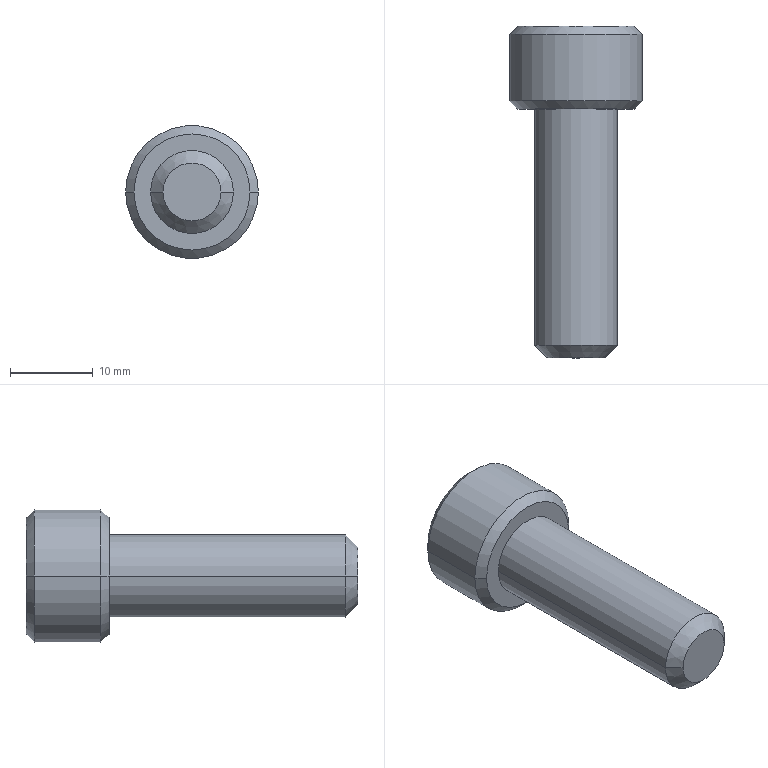Part | STEP file | BB62-M10-30L-9 | 1 solid | 27 faces | box 16 x 40 x 16 mm | volume 3957 mm3 | plane 15 | cone 8 | cylinder 4 | commonest cylinder face diameters 10 x2 16 x2
STEP:
#1=CARTESIAN_POINT('',(0.,2.359,0.));
#2=VERTEX_POINT('',#1);
#3=CARTESIAN_POINT('',(4.575,5.,0.));
#4=VERTEX_POINT('',#3);
#5=CARTESIAN_POINT('',(0.,2.359,0.));
#6=DIRECTION('',(0.866,0.5,0.));
#7=VECTOR('',#6,1000.);
#8=LINE('',#5,#7);
#9=EDGE_CURVE('',#2,#4,#8,.T.);
#10=ORIENTED_EDGE('',*,*,#9,.F.);
#11=CARTESIAN_POINT('',(-4.575,5.,0.));
#12=VERTEX_POINT('',#11);
#13=CARTESIAN_POINT('',(0.,2.359,0.));
#14=DIRECTION('',(-0.866,0.5,0.));
#15=VECTOR('',#14,1000.);
#16=LINE('',#13,#15);
#17=EDGE_CURVE('',#2,#12,#16,.T.);
#18=ORIENTED_EDGE('',*,*,#17,.T.);
#19=CARTESIAN_POINT('',(-3.962,5.,2.288));
#20=VERTEX_POINT('',#19);
#21=CARTESIAN_POINT('',(0.,5.,0.));
#22=DIRECTION('',(0.,-1.,0.));
#23=DIRECTION('',(-1.,0.,0.));
#24=AXIS2_PLACEMENT_3D('',#21,#22,#23);
#25=CIRCLE('',#24,4.575);
#26=EDGE_CURVE('',#20,#12,#25,.T.);
#27=ORIENTED_EDGE('',*,*,#26,.F.);
#28=CARTESIAN_POINT('',(0.,5.,4.575));
#29=VERTEX_POINT('',#28);
#30=CARTESIAN_POINT('',(0.,5.,0.));
#31=DIRECTION('',(0.,-1.,0.));
#32=DIRECTION('',(-1.,0.,0.));
#33=AXIS2_PLACEMENT_3D('',#30,#31,#32);
#34=CIRCLE('',#33,4.575);
#35=EDGE_CURVE('',#29,#20,#34,.T.);
#36=ORIENTED_EDGE('',*,*,#35,.F.);
#37=CARTESIAN_POINT('',(3.962,5.,2.287));
#38=VERTEX_POINT('',#37);
#39=CARTESIAN_POINT('',(0.,5.,0.));
#40=DIRECTION('',(0.,-1.,0.));
#41=DIRECTION('',(-1.,0.,0.));
#42=AXIS2_PLACEMENT_3D('',#39,#40,#41);
#43=CIRCLE('',#42,4.575);
#44=EDGE_CURVE('',#38,#29,#43,.T.);
#45=ORIENTED_EDGE('',*,*,#44,.F.);
#46=CARTESIAN_POINT('',(0.,5.,0.));
#47=DIRECTION('',(0.,-1.,0.));
#48=DIRECTION('',(-1.,0.,0.));
#49=AXIS2_PLACEMENT_3D('',#46,#47,#48);
#50=CIRCLE('',#49,4.575);
#51=EDGE_CURVE('',#4,#38,#50,.T.);
#52=ORIENTED_EDGE('',*,*,#51,.F.);
#53=EDGE_LOOP('',(#10,#18,#27,#36,#45,#52));
#54=FACE_OUTER_BOUND('',#53,.T.);
#55=CARTESIAN_POINT('',(0.,1002.359,0.));
#56=DIRECTION('',(0.,1.,0.));
#57=DIRECTION('',(1.,0.,0.));
#58=AXIS2_PLACEMENT_3D('',#55,#56,#57);
#59=CONICAL_SURFACE('',#58,1732.051,1.047);
#60=ADVANCED_FACE('',(#54),#59,.F.);
#61=CARTESIAN_POINT('',(3.5,-30.,0.));
#62=VERTEX_POINT('',#61);
#63=CARTESIAN_POINT('',(-3.5,-30.,0.));
#64=VERTEX_POINT('',#63);
#65=CARTESIAN_POINT('',(0.,-30.,0.));
#66=DIRECTION('',(0.,1.,0.));
#67=DIRECTION('',(1.,0.,0.));
#68=AXIS2_PLACEMENT_3D('',#65,#66,#67);
#69=CIRCLE('',#68,3.5);
#70=EDGE_CURVE('',#62,#64,#69,.T.);
#71=ORIENTED_EDGE('',*,*,#70,.T.);
#72=CARTESIAN_POINT('',(-5.,-28.5,0.));
#73=VERTEX_POINT('',#72);
#74=CARTESIAN_POINT('',(-3.5,-30.,0.));
#75=DIRECTION('',(-0.7071,0.7071,0.));
#76=VECTOR('',#75,1000.);
#77=LINE('',#74,#76);
#78=EDGE_CURVE('',#64,#73,#77,.T.);
#79=ORIENTED_EDGE('',*,*,#78,.T.);
#80=CARTESIAN_POINT('',(5.,-28.5,0.));
#81=VERTEX_POINT('',#80);
#82=CARTESIAN_POINT('',(0.,-28.5,0.));
#83=DIRECTION('',(0.,-1.,0.));
#84=DIRECTION('',(-1.,0.,0.));
#85=AXIS2_PLACEMENT_3D('',#82,#83,#84);
#86=CIRCLE('',#85,5.);
#87=EDGE_CURVE('',#73,#81,#86,.T.);
#88=ORIENTED_EDGE('',*,*,#87,.T.);
#89=CARTESIAN_POINT('',(3.5,-30.,0.));
#90=DIRECTION('',(0.7071,0.7071,0.));
#91=VECTOR('',#90,1000.);
#92=LINE('',#89,#91);
#93=EDGE_CURVE('',#62,#81,#92,.T.);
#94=ORIENTED_EDGE('',*,*,#93,.F.);
#95=EDGE_LOOP('',(#71,#79,#88,#94));
#96=FACE_OUTER_BOUND('',#95,.T.);
#97=CARTESIAN_POINT('',(0.,-30.,0.));
#98=DIRECTION('',(0.,1.,0.));
#99=DIRECTION('',(1.,0.,0.));
#100=AXIS2_PLACEMENT_3D('',#97,#98,#99);
#101=CONICAL_SURFACE('',#100,3.5,0.7854);
#102=ADVANCED_FACE('',(#96),#101,.T.);
#103=ORIENTED_EDGE('',*,*,#87,.F.);
#104=CARTESIAN_POINT('',(-5.,0.,0.));
#105=VERTEX_POINT('',#104);
#106=CARTESIAN_POINT('',(-5.,-28.5,0.));
#107=DIRECTION('',(0.,1.,0.));
#108=VECTOR('',#107,1000.);
#109=LINE('',#106,#108);
#110=EDGE_CURVE('',#73,#105,#109,.T.);
#111=ORIENTED_EDGE('',*,*,#110,.T.);
#112=CARTESIAN_POINT('',(5.,0.,0.));
#113=VERTEX_POINT('',#112);
#114=CARTESIAN_POINT('',(0.,0.,0.));
#115=DIRECTION('',(0.,-1.,0.));
#116=DIRECTION('',(-1.,0.,0.));
#117=AXIS2_PLACEMENT_3D('',#114,#115,#116);
#118=CIRCLE('',#117,5.);
#119=EDGE_CURVE('',#105,#113,#118,.T.);
#120=ORIENTED_EDGE('',*,*,#119,.T.);
#121=CARTESIAN_POINT('',(5.,-28.5,0.));
#122=DIRECTION('',(0.,1.,0.));
#123=VECTOR('',#122,1000.);
#124=LINE('',#121,#123);
#125=EDGE_CURVE('',#81,#113,#124,.T.);
#126=ORIENTED_EDGE('',*,*,#125,.F.);
#127=EDGE_LOOP('',(#103,#111,#120,#126));
#128=FACE_OUTER_BOUND('',#127,.T.);
#129=CARTESIAN_POINT('',(0.,-28.5,0.));
#130=DIRECTION('',(0.,1.,0.));
#131=DIRECTION('',(1.,0.,0.));
#132=AXIS2_PLACEMENT_3D('',#129,#130,#131);
#133=CYLINDRICAL_SURFACE('',#132,5.);
#134=ADVANCED_FACE('',(#128),#133,.T.);
#135=CARTESIAN_POINT('',(-7.,10.,0.));
#136=VERTEX_POINT('',#135);
#137=CARTESIAN_POINT('',(7.,10.,0.));
#138=VERTEX_POINT('',#137);
#139=CARTESIAN_POINT('',(0.,10.,0.));
#140=DIRECTION('',(0.,-1.,0.));
#141=DIRECTION('',(-1.,0.,0.));
#142=AXIS2_PLACEMENT_3D('',#139,#140,#141);
#143=CIRCLE('',#142,7.);
#144=EDGE_CURVE('',#136,#138,#143,.T.);
#145=ORIENTED_EDGE('',*,*,#144,.T.);
#146=CARTESIAN_POINT('',(8.,9.,0.));
#147=VERTEX_POINT('',#146);
#148=CARTESIAN_POINT('',(8.,9.,0.));
#149=DIRECTION('',(0.7071,-0.7071,0.));
#150=VECTOR('',#149,1000.);
#151=LINE('',#148,#150);
#152=EDGE_CURVE('',#138,#147,#151,.T.);
#153=ORIENTED_EDGE('',*,*,#152,.T.);
#154=CARTESIAN_POINT('',(-8.,9.,0.));
#155=VERTEX_POINT('',#154);
#156=CARTESIAN_POINT('',(0.,9.,0.));
#157=DIRECTION('',(0.,-1.,0.));
#158=DIRECTION('',(-1.,0.,0.));
#159=AXIS2_PLACEMENT_3D('',#156,#157,#158);
#160=CIRCLE('',#159,8.);
#161=EDGE_CURVE('',#155,#147,#160,.T.);
#162=ORIENTED_EDGE('',*,*,#161,.F.);
#163=CARTESIAN_POINT('',(-8.,9.,0.));
#164=DIRECTION('',(-0.7071,-0.7071,0.));
#165=VECTOR('',#164,1000.);
#166=LINE('',#163,#165);
#167=EDGE_CURVE('',#136,#155,#166,.T.);
#168=ORIENTED_EDGE('',*,*,#167,.F.);
#169=EDGE_LOOP('',(#145,#153,#162,#168));
#170=FACE_OUTER_BOUND('',#169,.T.);
#171=CARTESIAN_POINT('',(0.,9.,0.));
#172=DIRECTION('',(0.,-1.,0.));
#173=DIRECTION('',(-1.,0.,0.));
#174=AXIS2_PLACEMENT_3D('',#171,#172,#173);
#175=CONICAL_SURFACE('',#174,8.,0.7854);
#176=ADVANCED_FACE('',(#170),#175,.T.);
#177=ORIENTED_EDGE('',*,*,#161,.T.);
#178=CARTESIAN_POINT('',(8.,1.,0.));
#179=VERTEX_POINT('',#178);
#180=CARTESIAN_POINT('',(8.,1.62,0.));
#181=DIRECTION('',(0.,-1.,0.));
#182=VECTOR('',#181,1000.);
#183=LINE('',#180,#182);
#184=EDGE_CURVE('',#147,#179,#183,.T.);
#185=ORIENTED_EDGE('',*,*,#184,.T.);
#186=CARTESIAN_POINT('',(-8.,1.,0.));
#187=VERTEX_POINT('',#186);
#188=CARTESIAN_POINT('',(0.,1.,0.));
#189=DIRECTION('',(0.,-1.,0.));
#190=DIRECTION('',(-1.,0.,0.));
#191=AXIS2_PLACEMENT_3D('',#188,#189,#190);
#192=CIRCLE('',#191,8.);
#193=EDGE_CURVE('',#187,#179,#192,.T.);
#194=ORIENTED_EDGE('',*,*,#193,.F.);
#195=CARTESIAN_POINT('',(-8.,1.62,0.));
#196=DIRECTION('',(0.,-1.,0.));
#197=VECTOR('',#196,1000.);
#198=LINE('',#195,#197);
#199=EDGE_CURVE('',#155,#187,#198,.T.);
#200=ORIENTED_EDGE('',*,*,#199,.F.);
#201=EDGE_LOOP('',(#177,#185,#194,#200));
#202=FACE_OUTER_BOUND('',#201,.T.);
#203=CARTESIAN_POINT('',(0.,1.62,0.));
#204=DIRECTION('',(0.,-1.,0.));
#205=DIRECTION('',(-1.,0.,0.));
#206=AXIS2_PLACEMENT_3D('',#203,#204,#205);
#207=CYLINDRICAL_SURFACE('',#206,8.);
#208=ADVANCED_FACE('',(#202),#207,.T.);
#209=CARTESIAN_POINT('',(-7.,0.,0.));
#210=VERTEX_POINT('',#209);
#211=CARTESIAN_POINT('',(7.,0.,0.));
#212=VERTEX_POINT('',#211);
#213=CARTESIAN_POINT('',(0.,0.,0.));
#214=DIRECTION('',(0.,-1.,0.));
#215=DIRECTION('',(-1.,0.,0.));
#216=AXIS2_PLACEMENT_3D('',#213,#214,#215);
#217=CIRCLE('',#216,7.);
#218=EDGE_CURVE('',#210,#212,#217,.T.);
#219=ORIENTED_EDGE('',*,*,#218,.F.);
#220=CARTESIAN_POINT('',(-7.,0.,0.));
#221=DIRECTION('',(-0.7071,0.7071,0.));
#222=VECTOR('',#221,1000.);
#223=LINE('',#220,#222);
#224=EDGE_CURVE('',#210,#187,#223,.T.);
#225=ORIENTED_EDGE('',*,*,#224,.T.);
#226=ORIENTED_EDGE('',*,*,#193,.T.);
#227=CARTESIAN_POINT('',(7.,0.,0.));
#228=DIRECTION('',(0.7071,0.7071,0.));
#229=VECTOR('',#228,1000.);
#230=LINE('',#227,#229);
#231=EDGE_CURVE('',#212,#179,#230,.T.);
#232=ORIENTED_EDGE('',*,*,#231,.F.);
#233=EDGE_LOOP('',(#219,#225,#226,#232));
#234=FACE_OUTER_BOUND('',#233,.T.);
#235=CARTESIAN_POINT('',(0.,0.,0.));
#236=DIRECTION('',(0.,1.,0.));
#237=DIRECTION('',(1.,0.,0.));
#238=AXIS2_PLACEMENT_3D('',#235,#236,#237);
#239=CONICAL_SURFACE('',#238,7.,0.7854);
#240=ADVANCED_FACE('',(#234),#239,.T.);
#241=ORIENTED_EDGE('',*,*,#144,.F.);
#242=CARTESIAN_POINT('',(0.,10.,0.));
#243=DIRECTION('',(0.,-1.,0.));
#244=DIRECTION('',(-1.,0.,0.));
#245=AXIS2_PLACEMENT_3D('',#242,#243,#244);
#246=CIRCLE('',#245,7.);
#247=EDGE_CURVE('',#138,#136,#246,.T.);
#248=ORIENTED_EDGE('',*,*,#247,.F.);
#249=EDGE_LOOP('',(#241,#248));
#250=FACE_OUTER_BOUND('',#249,.T.);
#251=CARTESIAN_POINT('',(0.,10.,-4.575));
#252=VERTEX_POINT('',#251);
#253=CARTESIAN_POINT('',(-3.962,10.,-2.288));
#254=VERTEX_POINT('',#253);
#255=CARTESIAN_POINT('',(0.,10.,-4.575));
#256=DIRECTION('',(-0.866,0.,0.5));
#257=VECTOR('',#256,1000.);
#258=LINE('',#255,#257);
#259=EDGE_CURVE('',#252,#254,#258,.T.);
#260=ORIENTED_EDGE('',*,*,#259,.F.);
#261=CARTESIAN_POINT('',(3.962,10.,-2.288));
#262=VERTEX_POINT('',#261);
#263=CARTESIAN_POINT('',(3.962,10.,-2.288));
#264=DIRECTION('',(-0.866,0.,-0.5));
#265=VECTOR('',#264,1000.);
#266=LINE('',#263,#265);
#267=EDGE_CURVE('',#262,#252,#266,.T.);
#268=ORIENTED_EDGE('',*,*,#267,.F.);
#269=CARTESIAN_POINT('',(3.962,10.,2.287));
#270=VERTEX_POINT('',#269);
#271=CARTESIAN_POINT('',(3.962,10.,2.287));
#272=DIRECTION('',(0.,0.,-1.));
#273=VECTOR('',#272,1000.);
#274=LINE('',#271,#273);
#275=EDGE_CURVE('',#270,#262,#274,.T.);
#276=ORIENTED_EDGE('',*,*,#275,.F.);
#277=CARTESIAN_POINT('',(0.,10.,4.575));
#278=VERTEX_POINT('',#277);
#279=CARTESIAN_POINT('',(0.,10.,4.575));
#280=DIRECTION('',(0.866,0.,-0.5));
#281=VECTOR('',#280,1000.);
#282=LINE('',#279,#281);
#283=EDGE_CURVE('',#278,#270,#282,.T.);
#284=ORIENTED_EDGE('',*,*,#283,.F.);
#285=CARTESIAN_POINT('',(-3.962,10.,2.287));
#286=VERTEX_POINT('',#285);
#287=CARTESIAN_POINT('',(-3.962,10.,2.287));
#288=DIRECTION('',(0.866,0.,0.5));
#289=VECTOR('',#288,1000.);
#290=LINE('',#287,#289);
#291=EDGE_CURVE('',#286,#278,#290,.T.);
#292=ORIENTED_EDGE('',*,*,#291,.F.);
#293=CARTESIAN_POINT('',(-3.962,10.,-2.288));
#294=DIRECTION('',(0.,0.,1.));
#295=VECTOR('',#294,1000.);
#296=LINE('',#293,#295);
#297=EDGE_CURVE('',#254,#286,#296,.T.);
#298=ORIENTED_EDGE('',*,*,#297,.F.);
#299=EDGE_LOOP('',(#260,#268,#276,#284,#292,#298));
#300=FACE_BOUND('',#299,.T.);
#301=CARTESIAN_POINT('',(7.,10.,0.));
#302=DIRECTION('',(0.,1.,0.));
#303=DIRECTION('',(1.,0.,0.));
#304=AXIS2_PLACEMENT_3D('',#301,#302,#303);
#305=PLANE('',#304);
#306=ADVANCED_FACE('',(#250,#300),#305,.T.);
#307=CARTESIAN_POINT('',(0.,0.,0.));
#308=DIRECTION('',(0.,-1.,0.));
#309=DIRECTION('',(-1.,0.,0.));
#310=AXIS2_PLACEMENT_3D('',#307,#308,#309);
#311=CIRCLE('',#310,5.);
#312=EDGE_CURVE('',#113,#105,#311,.T.);
#313=ORIENTED_EDGE('',*,*,#312,.F.);
#314=ORIENTED_EDGE('',*,*,#119,.F.);
#315=EDGE_LOOP('',(#313,#314));
#316=FACE_BOUND('',#315,.T.);
#317=CARTESIAN_POINT('',(0.,0.,0.));
#318=DIRECTION('',(0.,-1.,0.));
#319=DIRECTION('',(-1.,0.,0.));
#320=AXIS2_PLACEMENT_3D('',#317,#318,#319);
#321=CIRCLE('',#320,7.);
#322=EDGE_CURVE('',#212,#210,#321,.T.);
#323=ORIENTED_EDGE('',*,*,#322,.T.);
#324=ORIENTED_EDGE('',*,*,#218,.T.);
#325=EDGE_LOOP('',(#323,#324));
#326=FACE_OUTER_BOUND('',#325,.T.);
#327=CARTESIAN_POINT('',(0.,0.,0.));
#328=DIRECTION('',(0.,-1.,0.));
#329=DIRECTION('',(-1.,0.,0.));
#330=AXIS2_PLACEMENT_3D('',#327,#328,#329);
#331=PLANE('',#330);
#332=ADVANCED_FACE('',(#316,#326),#331,.T.);
#333=ORIENTED_EDGE('',*,*,#224,.F.);
#334=ORIENTED_EDGE('',*,*,#322,.F.);
#335=ORIENTED_EDGE('',*,*,#231,.T.);
#336=CARTESIAN_POINT('',(0.,1.,0.));
#337=DIRECTION('',(0.,-1.,0.));
#338=DIRECTION('',(-1.,0.,0.));
#339=AXIS2_PLACEMENT_3D('',#336,#337,#338);
#340=CIRCLE('',#339,8.);
#341=EDGE_CURVE('',#179,#187,#340,.T.);
#342=ORIENTED_EDGE('',*,*,#341,.T.);
#343=EDGE_LOOP('',(#333,#334,#335,#342));
#344=FACE_OUTER_BOUND('',#343,.T.);
#345=CARTESIAN_POINT('',(0.,0.,0.));
#346=DIRECTION('',(0.,1.,0.));
#347=DIRECTION('',(1.,0.,0.));
#348=AXIS2_PLACEMENT_3D('',#345,#346,#347);
#349=CONICAL_SURFACE('',#348,7.,0.7854);
#350=ADVANCED_FACE('',(#344),#349,.T.);
#351=ORIENTED_EDGE('',*,*,#184,.F.);
#352=CARTESIAN_POINT('',(0.,9.,0.));
#353=DIRECTION('',(0.,-1.,0.));
#354=DIRECTION('',(-1.,0.,0.));
#355=AXIS2_PLACEMENT_3D('',#352,#353,#354);
#356=CIRCLE('',#355,8.);
#357=EDGE_CURVE('',#147,#155,#356,.T.);
#358=ORIENTED_EDGE('',*,*,#357,.T.);
#359=ORIENTED_EDGE('',*,*,#199,.T.);
#360=ORIENTED_EDGE('',*,*,#341,.F.);
#361=EDGE_LOOP('',(#351,#358,#359,#360));
#362=FACE_OUTER_BOUND('',#361,.T.);
#363=CARTESIAN_POINT('',(0.,1.62,0.));
#364=DIRECTION('',(0.,-1.,0.));
#365=DIRECTION('',(-1.,0.,0.));
#366=AXIS2_PLACEMENT_3D('',#363,#364,#365);
#367=CYLINDRICAL_SURFACE('',#366,8.);
#368=ADVANCED_FACE('',(#362),#367,.T.);
#369=ORIENTED_EDGE('',*,*,#152,.F.);
#370=ORIENTED_EDGE('',*,*,#247,.T.);
#371=ORIENTED_EDGE('',*,*,#167,.T.);
#372=ORIENTED_EDGE('',*,*,#357,.F.);
#373=EDGE_LOOP('',(#369,#370,#371,#372));
#374=FACE_OUTER_BOUND('',#373,.T.);
#375=CARTESIAN_POINT('',(0.,9.,0.));
#376=DIRECTION('',(0.,-1.,0.));
#377=DIRECTION('',(-1.,0.,0.));
#378=AXIS2_PLACEMENT_3D('',#375,#376,#377);
#379=CONICAL_SURFACE('',#378,8.,0.7854);
#380=ADVANCED_FACE('',(#374),#379,.T.);
#381=ORIENTED_EDGE('',*,*,#110,.F.);
#382=CARTESIAN_POINT('',(0.,-28.5,0.));
#383=DIRECTION('',(0.,-1.,0.));
#384=DIRECTION('',(-1.,0.,0.));
#385=AXIS2_PLACEMENT_3D('',#382,#383,#384);
#386=CIRCLE('',#385,5.);
#387=EDGE_CURVE('',#81,#73,#386,.T.);
#388=ORIENTED_EDGE('',*,*,#387,.F.);
#389=ORIENTED_EDGE('',*,*,#125,.T.);
#390=ORIENTED_EDGE('',*,*,#312,.T.);
#391=EDGE_LOOP('',(#381,#388,#389,#390));
#392=FACE_OUTER_BOUND('',#391,.T.);
#393=CARTESIAN_POINT('',(0.,-28.5,0.));
#394=DIRECTION('',(0.,1.,0.));
#395=DIRECTION('',(1.,0.,0.));
#396=AXIS2_PLACEMENT_3D('',#393,#394,#395);
#397=CYLINDRICAL_SURFACE('',#396,5.);
#398=ADVANCED_FACE('',(#392),#397,.T.);
#399=ORIENTED_EDGE('',*,*,#70,.F.);
#400=CARTESIAN_POINT('',(0.,-30.,0.));
#401=DIRECTION('',(0.,1.,0.));
#402=DIRECTION('',(1.,0.,0.));
#403=AXIS2_PLACEMENT_3D('',#400,#401,#402);
#404=CIRCLE('',#403,3.5);
#405=EDGE_CURVE('',#64,#62,#404,.T.);
#406=ORIENTED_EDGE('',*,*,#405,.F.);
#407=EDGE_LOOP('',(#399,#406));
#408=FACE_OUTER_BOUND('',#407,.T.);
#409=CARTESIAN_POINT('',(0.,-30.,0.));
#410=DIRECTION('',(0.,-1.,0.));
#411=DIRECTION('',(-1.,0.,0.));
#412=AXIS2_PLACEMENT_3D('',#409,#410,#411);
#413=PLANE('',#412);
#414=ADVANCED_FACE('',(#408),#413,.T.);
#415=ORIENTED_EDGE('',*,*,#78,.F.);
#416=ORIENTED_EDGE('',*,*,#405,.T.);
#417=ORIENTED_EDGE('',*,*,#93,.T.);
#418=ORIENTED_EDGE('',*,*,#387,.T.);
#419=EDGE_LOOP('',(#415,#416,#417,#418));
#420=FACE_OUTER_BOUND('',#419,.T.);
#421=CARTESIAN_POINT('',(0.,-30.,0.));
#422=DIRECTION('',(0.,1.,0.));
#423=DIRECTION('',(1.,0.,0.));
#424=AXIS2_PLACEMENT_3D('',#421,#422,#423);
#425=CONICAL_SURFACE('',#424,3.5,0.7854);
#426=ADVANCED_FACE('',(#420),#425,.T.);
#427=CARTESIAN_POINT('',(3.962,5.,-2.288));
#428=VERTEX_POINT('',#427);
#429=CARTESIAN_POINT('',(0.,5.,-4.575));
#430=VERTEX_POINT('',#429);
#431=CARTESIAN_POINT('',(3.962,5.,-2.288));
#432=DIRECTION('',(-0.866,0.,-0.5));
#433=VECTOR('',#432,1000.);
#434=LINE('',#431,#433);
#435=EDGE_CURVE('',#428,#430,#434,.T.);
#436=ORIENTED_EDGE('',*,*,#435,.F.);
#437=CARTESIAN_POINT('',(3.962,10.,-2.288));
#438=DIRECTION('',(0.,-1.,0.));
#439=VECTOR('',#438,1000.);
#440=LINE('',#437,#439);
#441=EDGE_CURVE('',#262,#428,#440,.T.);
#442=ORIENTED_EDGE('',*,*,#441,.F.);
#443=ORIENTED_EDGE('',*,*,#267,.T.);
#444=CARTESIAN_POINT('',(0.,10.,-4.575));
#445=DIRECTION('',(0.,-1.,0.));
#446=VECTOR('',#445,1000.);
#447=LINE('',#444,#446);
#448=EDGE_CURVE('',#252,#430,#447,.T.);
#449=ORIENTED_EDGE('',*,*,#448,.T.);
#450=EDGE_LOOP('',(#436,#442,#443,#449));
#451=FACE_OUTER_BOUND('',#450,.T.);
#452=CARTESIAN_POINT('',(3.962,10.,-2.288));
#453=DIRECTION('',(-0.5,0.,0.866));
#454=DIRECTION('',(0.866,0.,0.5));
#455=AXIS2_PLACEMENT_3D('',#452,#453,#454);
#456=PLANE('',#455);
#457=ADVANCED_FACE('',(#451),#456,.T.);
#458=CARTESIAN_POINT('',(-3.962,5.,-2.288));
#459=VERTEX_POINT('',#458);
#460=CARTESIAN_POINT('',(0.,5.,-4.575));
#461=DIRECTION('',(-0.866,0.,0.5));
#462=VECTOR('',#461,1000.);
#463=LINE('',#460,#462);
#464=EDGE_CURVE('',#430,#459,#463,.T.);
#465=ORIENTED_EDGE('',*,*,#464,.F.);
#466=ORIENTED_EDGE('',*,*,#448,.F.);
#467=ORIENTED_EDGE('',*,*,#259,.T.);
#468=CARTESIAN_POINT('',(-3.962,10.,-2.288));
#469=DIRECTION('',(0.,-1.,0.));
#470=VECTOR('',#469,1000.);
#471=LINE('',#468,#470);
#472=EDGE_CURVE('',#254,#459,#471,.T.);
#473=ORIENTED_EDGE('',*,*,#472,.T.);
#474=EDGE_LOOP('',(#465,#466,#467,#473));
#475=FACE_OUTER_BOUND('',#474,.T.);
#476=CARTESIAN_POINT('',(0.,10.,-4.575));
#477=DIRECTION('',(0.5,0.,0.866));
#478=DIRECTION('',(0.866,0.,-0.5));
#479=AXIS2_PLACEMENT_3D('',#476,#477,#478);
#480=PLANE('',#479);
#481=ADVANCED_FACE('',(#475),#480,.T.);
#482=CARTESIAN_POINT('',(-3.962,5.,-2.288));
#483=DIRECTION('',(0.,0.,1.));
#484=VECTOR('',#483,1000.);
#485=LINE('',#482,#484);
#486=EDGE_CURVE('',#459,#20,#485,.T.);
#487=ORIENTED_EDGE('',*,*,#486,.F.);
#488=ORIENTED_EDGE('',*,*,#472,.F.);
#489=ORIENTED_EDGE('',*,*,#297,.T.);
#490=CARTESIAN_POINT('',(-3.962,10.,2.287));
#491=DIRECTION('',(0.,-1.,0.));
#492=VECTOR('',#491,1000.);
#493=LINE('',#490,#492);
#494=EDGE_CURVE('',#286,#20,#493,.T.);
#495=ORIENTED_EDGE('',*,*,#494,.T.);
#496=EDGE_LOOP('',(#487,#488,#489,#495));
#497=FACE_OUTER_BOUND('',#496,.T.);
#498=CARTESIAN_POINT('',(-3.962,10.,-2.288));
#499=DIRECTION('',(1.,0.,0.));
#500=DIRECTION('',(0.,0.,-1.));
#501=AXIS2_PLACEMENT_3D('',#498,#499,#500);
#502=PLANE('',#501);
#503=ADVANCED_FACE('',(#497),#502,.T.);
#504=CARTESIAN_POINT('',(-3.962,5.,2.287));
#505=DIRECTION('',(0.866,0.,0.5));
#506=VECTOR('',#505,1000.);
#507=LINE('',#504,#506);
#508=EDGE_CURVE('',#20,#29,#507,.T.);
#509=ORIENTED_EDGE('',*,*,#508,.F.);
#510=ORIENTED_EDGE('',*,*,#494,.F.);
#511=ORIENTED_EDGE('',*,*,#291,.T.);
#512=CARTESIAN_POINT('',(0.,10.,4.575));
#513=DIRECTION('',(0.,-1.,0.));
#514=VECTOR('',#513,1000.);
#515=LINE('',#512,#514);
#516=EDGE_CURVE('',#278,#29,#515,.T.);
#517=ORIENTED_EDGE('',*,*,#516,.T.);
#518=EDGE_LOOP('',(#509,#510,#511,#517));
#519=FACE_OUTER_BOUND('',#518,.T.);
#520=CARTESIAN_POINT('',(-3.962,10.,2.287));
#521=DIRECTION('',(0.5,0.,-0.866));
#522=DIRECTION('',(-0.866,0.,-0.5));
#523=AXIS2_PLACEMENT_3D('',#520,#521,#522);
#524=PLANE('',#523);
#525=ADVANCED_FACE('',(#519),#524,.T.);
#526=CARTESIAN_POINT('',(0.,5.,4.575));
#527=DIRECTION('',(0.866,0.,-0.5));
#528=VECTOR('',#527,1000.);
#529=LINE('',#526,#528);
#530=EDGE_CURVE('',#29,#38,#529,.T.);
#531=ORIENTED_EDGE('',*,*,#530,.F.);
#532=ORIENTED_EDGE('',*,*,#516,.F.);
#533=ORIENTED_EDGE('',*,*,#283,.T.);
#534=CARTESIAN_POINT('',(3.962,10.,2.287));
#535=DIRECTION('',(0.,-1.,0.));
#536=VECTOR('',#535,1000.);
#537=LINE('',#534,#536);
#538=EDGE_CURVE('',#270,#38,#537,.T.);
#539=ORIENTED_EDGE('',*,*,#538,.T.);
#540=EDGE_LOOP('',(#531,#532,#533,#539));
#541=FACE_OUTER_BOUND('',#540,.T.);
#542=CARTESIAN_POINT('',(0.,10.,4.575));
#543=DIRECTION('',(-0.5,0.,-0.866));
#544=DIRECTION('',(-0.866,0.,0.5));
#545=AXIS2_PLACEMENT_3D('',#542,#543,#544);
#546=PLANE('',#545);
#547=ADVANCED_FACE('',(#541),#546,.T.);
#548=CARTESIAN_POINT('',(3.962,5.,2.287));
#549=DIRECTION('',(0.,0.,-1.));
#550=VECTOR('',#549,1000.);
#551=LINE('',#548,#550);
#552=EDGE_CURVE('',#38,#428,#551,.T.);
#553=ORIENTED_EDGE('',*,*,#552,.F.);
#554=ORIENTED_EDGE('',*,*,#538,.F.);
#555=ORIENTED_EDGE('',*,*,#275,.T.);
#556=ORIENTED_EDGE('',*,*,#441,.T.);
#557=EDGE_LOOP('',(#553,#554,#555,#556));
#558=FACE_OUTER_BOUND('',#557,.T.);
#559=CARTESIAN_POINT('',(3.962,10.,2.287));
#560=DIRECTION('',(-1.,0.,0.));
#561=DIRECTION('',(0.,0.,1.));
#562=AXIS2_PLACEMENT_3D('',#559,#560,#561);
#563=PLANE('',#562);
#564=ADVANCED_FACE('',(#558),#563,.T.);
#565=ORIENTED_EDGE('',*,*,#435,.T.);
#566=CARTESIAN_POINT('',(0.,5.,0.));
#567=DIRECTION('',(0.,-1.,0.));
#568=DIRECTION('',(-1.,0.,0.));
#569=AXIS2_PLACEMENT_3D('',#566,#567,#568);
#570=CIRCLE('',#569,4.575);
#571=EDGE_CURVE('',#430,#428,#570,.T.);
#572=ORIENTED_EDGE('',*,*,#571,.T.);
#573=EDGE_LOOP('',(#565,#572));
#574=FACE_OUTER_BOUND('',#573,.T.);
#575=CARTESIAN_POINT('',(0.,5.,0.));
#576=DIRECTION('',(0.,1.,0.));
#577=DIRECTION('',(1.,0.,0.));
#578=AXIS2_PLACEMENT_3D('',#575,#576,#577);
#579=PLANE('',#578);
#580=ADVANCED_FACE('',(#574),#579,.F.);
#581=ORIENTED_EDGE('',*,*,#552,.T.);
#582=CARTESIAN_POINT('',(0.,5.,0.));
#583=DIRECTION('',(0.,-1.,0.));
#584=DIRECTION('',(-1.,0.,0.));
#585=AXIS2_PLACEMENT_3D('',#582,#583,#584);
#586=CIRCLE('',#585,4.575);
#587=EDGE_CURVE('',#428,#4,#586,.T.);
#588=ORIENTED_EDGE('',*,*,#587,.T.);
#589=ORIENTED_EDGE('',*,*,#51,.T.);
#590=EDGE_LOOP('',(#581,#588,#589));
#591=FACE_OUTER_BOUND('',#590,.T.);
#592=CARTESIAN_POINT('',(0.,5.,0.));
#593=DIRECTION('',(0.,1.,0.));
#594=DIRECTION('',(1.,0.,0.));
#595=AXIS2_PLACEMENT_3D('',#592,#593,#594);
#596=PLANE('',#595);
#597=ADVANCED_FACE('',(#591),#596,.F.);
#598=ORIENTED_EDGE('',*,*,#530,.T.);
#599=ORIENTED_EDGE('',*,*,#44,.T.);
#600=EDGE_LOOP('',(#598,#599));
#601=FACE_OUTER_BOUND('',#600,.T.);
#602=CARTESIAN_POINT('',(0.,5.,0.));
#603=DIRECTION('',(0.,1.,0.));
#604=DIRECTION('',(1.,0.,0.));
#605=AXIS2_PLACEMENT_3D('',#602,#603,#604);
#606=PLANE('',#605);
#607=ADVANCED_FACE('',(#601),#606,.F.);
#608=ORIENTED_EDGE('',*,*,#508,.T.);
#609=ORIENTED_EDGE('',*,*,#35,.T.);
#610=EDGE_LOOP('',(#608,#609));
#611=FACE_OUTER_BOUND('',#610,.T.);
#612=CARTESIAN_POINT('',(0.,5.,0.));
#613=DIRECTION('',(0.,1.,0.));
#614=DIRECTION('',(1.,0.,0.));
#615=AXIS2_PLACEMENT_3D('',#612,#613,#614);
#616=PLANE('',#615);
#617=ADVANCED_FACE('',(#611),#616,.F.);
#618=ORIENTED_EDGE('',*,*,#486,.T.);
#619=ORIENTED_EDGE('',*,*,#26,.T.);
#620=CARTESIAN_POINT('',(0.,5.,0.));
#621=DIRECTION('',(0.,-1.,0.));
#622=DIRECTION('',(-1.,0.,0.));
#623=AXIS2_PLACEMENT_3D('',#620,#621,#622);
#624=CIRCLE('',#623,4.575);
#625=EDGE_CURVE('',#12,#459,#624,.T.);
#626=ORIENTED_EDGE('',*,*,#625,.T.);
#627=EDGE_LOOP('',(#618,#619,#626));
#628=FACE_OUTER_BOUND('',#627,.T.);
#629=CARTESIAN_POINT('',(0.,5.,0.));
#630=DIRECTION('',(0.,1.,0.));
#631=DIRECTION('',(1.,0.,0.));
#632=AXIS2_PLACEMENT_3D('',#629,#630,#631);
#633=PLANE('',#632);
#634=ADVANCED_FACE('',(#628),#633,.F.);
#635=ORIENTED_EDGE('',*,*,#464,.T.);
#636=CARTESIAN_POINT('',(0.,5.,0.));
#637=DIRECTION('',(0.,-1.,0.));
#638=DIRECTION('',(-1.,0.,0.));
#639=AXIS2_PLACEMENT_3D('',#636,#637,#638);
#640=CIRCLE('',#639,4.575);
#641=EDGE_CURVE('',#459,#430,#640,.T.);
#642=ORIENTED_EDGE('',*,*,#641,.T.);
#643=EDGE_LOOP('',(#635,#642));
#644=FACE_OUTER_BOUND('',#643,.T.);
#645=CARTESIAN_POINT('',(0.,5.,0.));
#646=DIRECTION('',(0.,1.,0.));
#647=DIRECTION('',(1.,0.,0.));
#648=AXIS2_PLACEMENT_3D('',#645,#646,#647);
#649=PLANE('',#648);
#650=ADVANCED_FACE('',(#644),#649,.F.);
#651=ORIENTED_EDGE('',*,*,#17,.F.);
#652=ORIENTED_EDGE('',*,*,#9,.T.);
#653=ORIENTED_EDGE('',*,*,#587,.F.);
#654=ORIENTED_EDGE('',*,*,#571,.F.);
#655=ORIENTED_EDGE('',*,*,#641,.F.);
#656=ORIENTED_EDGE('',*,*,#625,.F.);
#657=EDGE_LOOP('',(#651,#652,#653,#654,#655,#656));
#658=FACE_OUTER_BOUND('',#657,.T.);
#659=CARTESIAN_POINT('',(0.,1002.359,0.));
#660=DIRECTION('',(0.,1.,0.));
#661=DIRECTION('',(1.,0.,0.));
#662=AXIS2_PLACEMENT_3D('',#659,#660,#661);
#663=CONICAL_SURFACE('',#662,1732.051,1.047);
#664=ADVANCED_FACE('',(#658),#663,.F.);
#665=CLOSED_SHELL('',(#60,#102,#134,#176,#208,#240,#306,#332,#350,#368,#380,#398,#414,#426,#457,#481,#503,#525,#547,#564,#580,#597,#607,#617,#634,#650,#664));
#666=MANIFOLD_SOLID_BREP('',#665);
#667=CARTESIAN_POINT('',(0.,0.,0.));
#668=DIRECTION('',(0.,0.,1.));
#669=DIRECTION('',(1.,0.,0.));
#670=AXIS2_PLACEMENT_3D('',#667,#668,#669);
#671=(LENGTH_UNIT()NAMED_UNIT(*)SI_UNIT(.MILLI.,.METRE.));
#672=UNCERTAINTY_MEASURE_WITH_UNIT(LENGTH_MEASURE(0.00001),#671,'','');
#673=(NAMED_UNIT(*)PLANE_ANGLE_UNIT()SI_UNIT($,.RADIAN.));
#674=(NAMED_UNIT(*)SI_UNIT($,.STERADIAN.)SOLID_ANGLE_UNIT());
#675=(GEOMETRIC_REPRESENTATION_CONTEXT(3)GLOBAL_UNCERTAINTY_ASSIGNED_CONTEXT((#672))GLOBAL_UNIT_ASSIGNED_CONTEXT((#671,#673,#674))REPRESENTATION_CONTEXT('',''));
#676=ADVANCED_BREP_SHAPE_REPRESENTATION('',(#666,#670),#675);